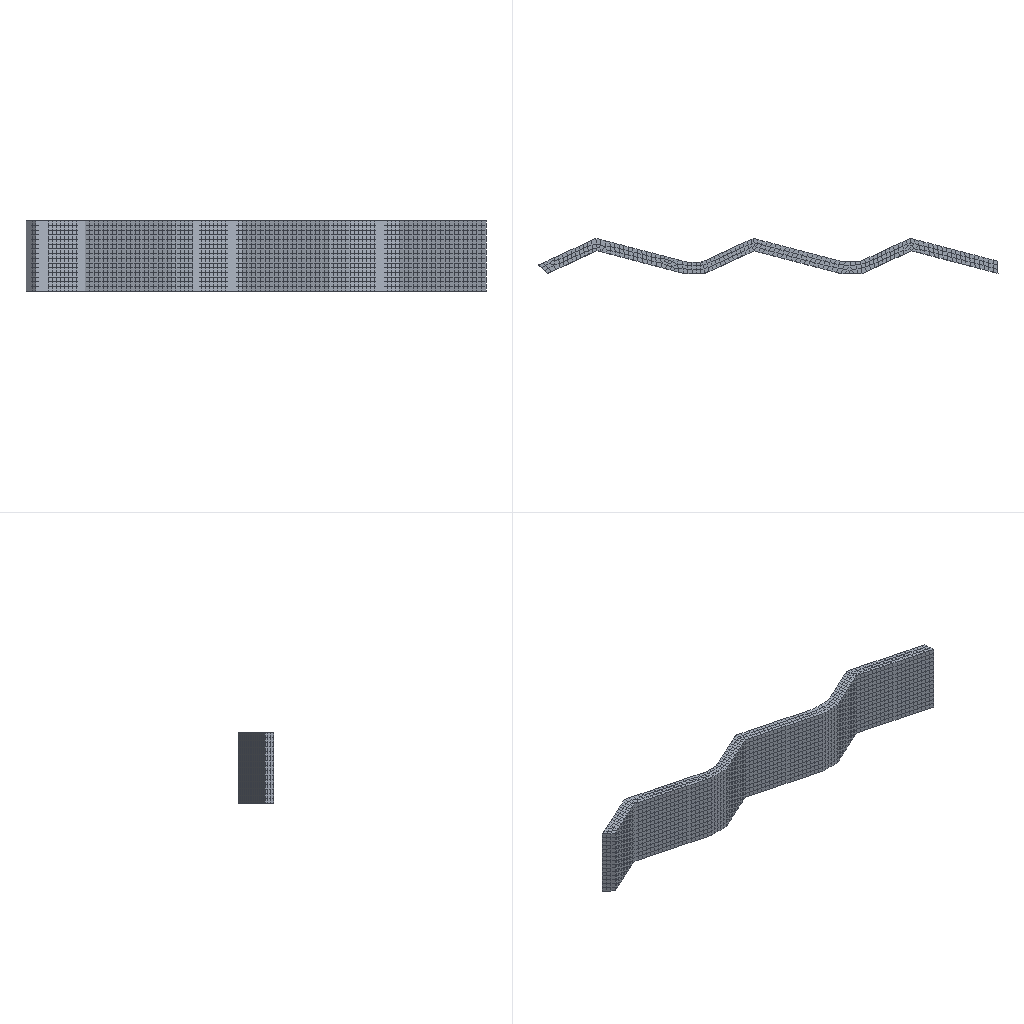Simulation study | abaqus
Set-up summary:
category,name,step,type,value,unit,region
solver,abaqus
solver,version,,,Abaqus/Explicit 2020
units,not stated in the deck,,not stated
analysis,deck,,transient,transient
load_step,Step-1,Step-1,transient
load_step,requested,,,1
mesh,nodes,,,9900
mesh,elements,,,7853
element_type,R3D3,,rigid,16
element_type,R3D4,,rigid,3022
element_type,C3D8R,,solid,4815
load,load commands in deck,,count,2
bc,support commands in deck,,count,7
material,MATERIAL-1,,in results
check,setup vs results,,match,"per instance, exact: element labels, types and connectivity; labels of the nodes the elements use; coordinates of those nodes at SINGLE_PRECISION in 1 of 3 instance(s)"
Abaqus input file, long lists of numbers shortened:
*Heading
** Job name: Job-1 Model name: Model-1
** Generated by: Abaqus/CAE 2020
*Preprint, echo=NO, model=NO, history=NO, contact=NO
**
** PARTS
**
*Part, name=Part-1
*Node
      1,           0.,           0.,          32.
      2,           6.,           0.,          32.
** (1515 more lines like these left out)
*Element, type=R3D4
1,  1,  2, 25, 38
2, 38, 25, 26, 37
** (1509 more lines like these left out)
*Element, type=R3D3
913, 1264, 1184, 1178
914, 1266, 1226, 1221
** (6 more lines like these left out)
*Node
   1518,   98.987,         -25.,          32.
*Nset, nset=Part-1-RefPt_, internal
1518,
*Elset, elset=Part-1, generate
    1,  1519,     1
*End Part
**
*Part, name=work
*Node
      1,   84.915,   6.268,           0.
      2,   89.055,   9.864,           0.
** (6862 more lines like these left out)
*Element, type=C3D8R
   1,   91,  393,   96,  246,  520,  822,  525,  675
   2,  275,  287,  135,  134,  704,  716,  564,  563
** (4813 more lines like these left out)
*Nset, nset=Set-2, generate
    1,  6864,     1
*Elset, elset=Set-2, generate
    1,  4815,     1
** Section: Section-1
*Solid Section, elset=Set-2, material=Material-1
,
*End Part
**
**
** ASSEMBLY
**
*Assembly, name=Assembly
**
*Instance, name=Part-1-1, part=Part-1
        -35.,           2.,           0.
*End Instance
**
*Instance, name=Part-1-2, part=Part-1
         -2.,           2.,          32.
         -2.,           2.,          32.,          -1.,           2.,          32.,         180.
*End Instance
**
*Instance, name=work-1, part=work
  -84.682,      6.598,          32.
  -84.682,      6.598,          32.,   -83.682,      6.598,          32.,         180.
*End Instance
**
*Nset, nset=Set-1, instance=Part-1-2
 1518,
*Nset, nset=Set-2, instance=Part-1-1
 1518,
*Nset, nset=Set-3, instance=work-1
   42,   43,  197,  198,  471,  472,  626,  627,  900,  901, 1055, 1056, 1329, 1330, 1484, 1485
 1758, 1759, 1913, 1914, 2187, 2188, 2342, 2343, 2616, 2617, 2771, 2772, 3045, 3046, 3200, 3201
** (2 more lines like these left out)
*Elset, elset=Set-3, instance=work-1
   96,  195,  196,  417,  516,  517,  738,  837,  838, 1059, 1158, 1159, 1380, 1479, 1480, 1701
 1800, 1801, 2022, 2121, 2122, 2343, 2442, 2443, 2664, 2763, 2764, 2985, 3084, 3085, 3306, 3405
** (1 more lines like these left out)
*Elset, elset=_Surf-5_S6, internal, instance=work-1
   96,  196,  417,  517,  738,  838, 1059, 1159, 1380, 1480, 1701, 1801, 2022, 2122, 2343, 2443
 2664, 2764, 2985, 3085, 3306, 3406, 3627, 3727, 3948, 4048, 4269, 4369, 4590, 4690
*Elset, elset=_Surf-5_S4, internal, instance=work-1, generate
  195,  4689,   321
*Surface, type=ELEMENT, name=Surf-5
_Surf-5_S6, S6
_Surf-5_S4, S4
*Elset, elset=_m_Surf-1_SPOS, internal, instance=Part-1-1, generate
  57,  424,    1
*Surface, type=ELEMENT, name=m_Surf-1
_m_Surf-1_SPOS, SPOS
*Elset, elset=_m_Surf-3_SPOS, internal, instance=Part-1-2, generate
   9,  424,    1
*Surface, type=ELEMENT, name=m_Surf-3
_m_Surf-3_SPOS, SPOS
*Elset, elset=_s_Surf-1_S5, internal, instance=work-1
    2,   48,   63,   91,   95,   97,   98,  100,  105,  107,  140,  156,  158,  162,  192,  194
  195,  265,  269,  279,  280,  283,  286,  293,  295,  296,  313,  323,  369,  384,  412,  416
** (24 more lines like these left out)
*Elset, elset=_s_Surf-1_S6, internal, instance=work-1
    3,    7,   18,   47,   51,   57,   64,   74,   83,   84,   85,  145,  146,  148,  160,  165
  167,  177,  178,  182,  183,  184,  185,  186,  191,  248,  249,  324,  328,  339,  368,  372
** (24 more lines like these left out)
*Elset, elset=_s_Surf-1_S4, internal, instance=work-1
    5,   28,   33,   34,   38,   62,   69,   82,  122,  139,  144,  150,  152,  159,  161,  164
  173,  175,  176,  180,  181,  187,  188,  189,  230,  231,  232,  233,  234,  236,  251,  257
** (37 more lines like these left out)
*Elset, elset=_s_Surf-1_S3, internal, instance=work-1
   17,   31,   40,  104,  106,  168,  193,  268,  338,  352,  361,  425,  427,  489,  514,  589
  659,  673,  682,  746,  748,  810,  835,  910,  980,  994, 1003, 1067, 1069, 1131, 1156, 1231
** (6 more lines like these left out)
*Surface, type=ELEMENT, name=s_Surf-1
_s_Surf-1_S5, S5
_s_Surf-1_S6, S6
_s_Surf-1_S4, S4
_s_Surf-1_S3, S3
*Elset, elset=_s_Surf-3_S5, internal, instance=work-1
   12,   22,   23,   35,   42,   60,   77,   79,  102,  110,  114,  118,  119,  129,  130,  138
  196,  207,  211,  213,  214,  216,  217,  218,  219,  245,  247,  271,  273,  274,  275,  278
** (36 more lines like these left out)
*Elset, elset=_s_Surf-3_S3, internal, instance=work-1
   11,   20,   21,   24,   43,   46,   50,   87,   89,   94,  109,  125,  126,  127,  128,  135
  137,  142,  143,  153,  154,  170,  197,  199,  212,  244,  258,  290,  291,  299,  301,  303
** (28 more lines like these left out)
*Elset, elset=_s_Surf-3_S4, internal, instance=work-1
   27,   88,  132,  134,  151,  201,  204,  205,  206,  220,  222,  227,  250,  255,  261,  262
  263,  308,  310,  317,  348,  409,  453,  455,  472,  522,  525,  526,  527,  541,  543,  548
** (17 more lines like these left out)
*Elset, elset=_s_Surf-3_S6, internal, instance=work-1
    1,   44,   45,   58,   71,  113,  131,  133,  200,  208,  210,  215,  221,  322,  365,  366
  379,  392,  434,  452,  454,  521,  529,  531,  536,  542,  643,  686,  687,  700,  713,  755
** (11 more lines like these left out)
*Surface, type=ELEMENT, name=s_Surf-3
_s_Surf-3_S5, S5
_s_Surf-3_S3, S3
_s_Surf-3_S4, S4
_s_Surf-3_S6, S6
*Rigid Body, ref node=Part-1-1.Part-1-RefPt_, elset=Part-1-1.Part-1
*Rigid Body, ref node=Part-1-2.Part-1-RefPt_, elset=Part-1-2.Part-1
** Constraint: Constraint-1
*Tie, name=Constraint-1, adjust=yes
s_Surf-1, m_Surf-1
** Constraint: Constraint-2
*Tie, name=Constraint-2, adjust=yes
s_Surf-3, m_Surf-3
*End Assembly
*Amplitude, name=Amp-1
             0.,              0.,             0.1,              1.
**
** MATERIALS
**
*Material, name=Material-1
*Density
 2.7e-09,
*Elastic
69000., 0.28
*Plastic
300.,0.
**
** INTERACTION PROPERTIES
**
*Surface Interaction, name=IntProp-1
*Friction
 0.2,
*Surface Behavior, pressure-overclosure=HARD
** ----------------------------------------------------------------
**
** STEP: Step-1
**
*Step, name=Step-1, nlgeom=YES
*Dynamic, Explicit
, 0.1
*Bulk Viscosity
0.06, 1.2
** Mass Scaling: Semi-Automatic
**               Whole Model
*Fixed Mass Scaling, factor=50.
**
** BOUNDARY CONDITIONS
**
** Name: BC-1 Type: 对称/反对称/完全固定
*Boundary
Set-1, ENCASTRE
** Name: BC-2 Type: 位移/转角
*Boundary, amplitude=Amp-1
Set-2, 1, 1
Set-2, 2, 2, 5.
Set-2, 3, 3
Set-2, 4, 4
Set-2, 5, 5
Set-2, 6, 6
**
** LOADS
**
** Name: Load-1   Type: Pressure
*Dsload
Surf-5, P, -5.
**
** INTERACTIONS
**
** Interaction: Int-1
*Contact, op=NEW
*Contact Inclusions, ALL EXTERIOR
*Contact Property Assignment
 ,  , IntProp-1
**
** OUTPUT REQUESTS
**
*Restart, write, number interval=1, time marks=NO
**
** FIELD OUTPUT: F-Output-1
**
*Output, field, number interval=50
*Node Output
A, RF, RM, RT, U, UR, UT, V
VR, VT
*Element Output, directions=YES
E, EVF, LE, MISES, MISESMAX, PE, PEEQ, PEEQVAVG, PEVAVG, S, SVAVG, VE
*Contact Output
CDISP, CSTRESS
**
** HISTORY OUTPUT: H-Output-1
**
*Output, history, variable=PRESELECT
*End Step
Results summary:
result,step,Step-1,completed,increments=97941 time=0.1/0.1
result,analysis,,,transient
result,last_loadstep,,,1
result,primary field,,,U
result,reaction total,,FX,-2178.453,model units
result,reaction total,,FY,911.0,model units
result,reaction total,,FZ,1421.324,model units